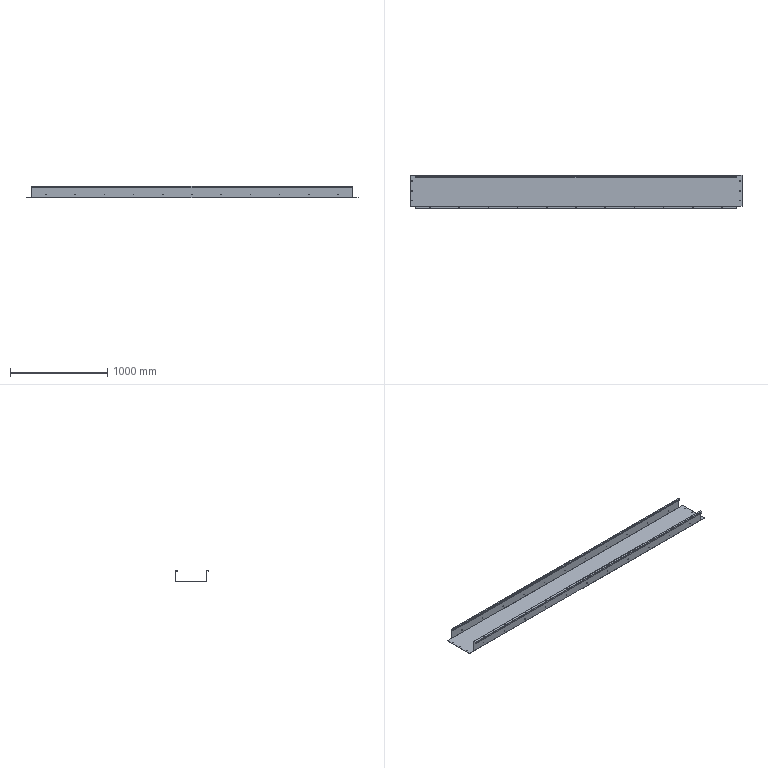Part | STEP file | SX-S02 | 1 solid | 192 faces | box 3411 x 343 x 122 mm | volume 4146327 mm3 | cylinder 112 | plane 80 | commonest cylinder face diameters 5.4 x66 8 x22 7 x12 0.4 x6 4.4 x6